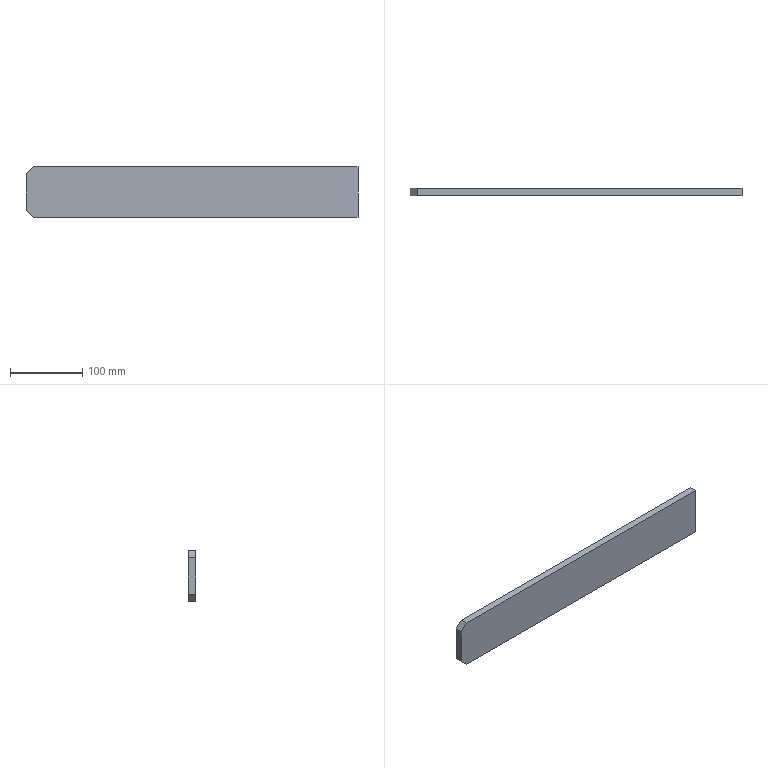Part | STEP file | Positioning_id1102_x_t | 1 solid | 8 faces | box 460 x 10 x 70 mm | volume 321000 mm3 | plane 8
STEP:
#1=CARTESIAN_POINT('',(0.,0.,0.));
#2=DIRECTION('',(0.,0.,1.));
#3=DIRECTION('',(1.,0.,0.));
#4=AXIS2_PLACEMENT_3D('',#1,#2,#3);
#5=CARTESIAN_POINT('',(-1483.002,800.,162.466));
#6=VERTEX_POINT('',#5);
#7=CARTESIAN_POINT('',(-1493.002,800.,172.466));
#8=VERTEX_POINT('',#7);
#9=CARTESIAN_POINT('',(-1483.002,800.,162.466));
#10=DIRECTION('',(-0.7071,0.,0.7071));
#11=VECTOR('',#10,1.);
#12=LINE('',#9,#11);
#13=CARTESIAN_POINT('',(-1493.002,800.,172.466));
#14=DIRECTION('',(0.7071,0.,0.7071));
#15=DIRECTION('',(-0.7071,0.,0.7071));
#16=AXIS2_PLACEMENT_3D('',#13,#14,#15);
#17=PLANE('',#16);
#18=CARTESIAN_POINT('',(-14.142,0.));
#19=DIRECTION('',(1.,0.));
#20=VECTOR('',#19,1.);
#21=LINE('',#18,#20);
#22=(GEOMETRIC_REPRESENTATION_CONTEXT(2)PARAMETRIC_REPRESENTATION_CONTEXT()REPRESENTATION_CONTEXT('',''));
#23=DEFINITIONAL_REPRESENTATION('',(#21),#22);
#24=PCURVE('',#17,#23);
#25=CARTESIAN_POINT('',(-1238.002,800.,197.466));
#26=DIRECTION('',(0.,-1.,0.));
#27=DIRECTION('',(0.,0.,1.));
#28=AXIS2_PLACEMENT_3D('',#25,#26,#27);
#29=PLANE('',#28);
#30=CARTESIAN_POINT('',(-35.,245.));
#31=DIRECTION('',(0.7071,0.7071));
#32=VECTOR('',#31,1.);
#33=LINE('',#30,#32);
#34=(GEOMETRIC_REPRESENTATION_CONTEXT(2)PARAMETRIC_REPRESENTATION_CONTEXT()REPRESENTATION_CONTEXT('',''));
#35=DEFINITIONAL_REPRESENTATION('',(#33),#34);
#36=PCURVE('',#29,#35);
#37=SURFACE_CURVE('',#12,(#24,#36),.PCURVE_S1.);
#38=EDGE_CURVE('',#6,#8,#37,.T.);
#39=ORIENTED_EDGE('',*,*,#38,.T.);
#40=CARTESIAN_POINT('',(-1493.002,810.,172.466));
#41=VERTEX_POINT('',#40);
#42=CARTESIAN_POINT('',(-1493.002,800.,172.466));
#43=DIRECTION('',(0.,1.,0.));
#44=VECTOR('',#43,1.);
#45=LINE('',#42,#44);
#46=CARTESIAN_POINT('',(0.,0.));
#47=DIRECTION('',(0.,-1.));
#48=VECTOR('',#47,1.);
#49=LINE('',#46,#48);
#50=(GEOMETRIC_REPRESENTATION_CONTEXT(2)PARAMETRIC_REPRESENTATION_CONTEXT()REPRESENTATION_CONTEXT('',''));
#51=DEFINITIONAL_REPRESENTATION('',(#49),#50);
#52=PCURVE('',#17,#51);
#53=CARTESIAN_POINT('',(-1493.002,800.,197.466));
#54=DIRECTION('',(-1.,0.,0.));
#55=DIRECTION('',(0.,-1.,0.));
#56=AXIS2_PLACEMENT_3D('',#53,#54,#55);
#57=PLANE('',#56);
#58=CARTESIAN_POINT('',(0.,-25.));
#59=DIRECTION('',(-1.,0.));
#60=VECTOR('',#59,1.);
#61=LINE('',#58,#60);
#62=(GEOMETRIC_REPRESENTATION_CONTEXT(2)PARAMETRIC_REPRESENTATION_CONTEXT()REPRESENTATION_CONTEXT('',''));
#63=DEFINITIONAL_REPRESENTATION('',(#61),#62);
#64=PCURVE('',#57,#63);
#65=SURFACE_CURVE('',#45,(#52,#64),.PCURVE_S1.);
#66=EDGE_CURVE('',#8,#41,#65,.T.);
#67=ORIENTED_EDGE('',*,*,#66,.T.);
#68=CARTESIAN_POINT('',(-1483.002,810.,162.466));
#69=VERTEX_POINT('',#68);
#70=CARTESIAN_POINT('',(-1493.002,810.,172.466));
#71=DIRECTION('',(0.7071,0.,-0.7071));
#72=VECTOR('',#71,1.);
#73=LINE('',#70,#72);
#74=CARTESIAN_POINT('',(0.,-10.));
#75=DIRECTION('',(-1.,0.));
#76=VECTOR('',#75,1.);
#77=LINE('',#74,#76);
#78=(GEOMETRIC_REPRESENTATION_CONTEXT(2)PARAMETRIC_REPRESENTATION_CONTEXT()REPRESENTATION_CONTEXT('',''));
#79=DEFINITIONAL_REPRESENTATION('',(#77),#78);
#80=PCURVE('',#17,#79);
#81=CARTESIAN_POINT('',(-1238.002,810.,197.466));
#82=DIRECTION('',(0.,1.,0.));
#83=DIRECTION('',(0.,0.,-1.));
#84=AXIS2_PLACEMENT_3D('',#81,#82,#83);
#85=PLANE('',#84);
#86=CARTESIAN_POINT('',(25.,255.));
#87=DIRECTION('',(0.7071,-0.7071));
#88=VECTOR('',#87,1.);
#89=LINE('',#86,#88);
#90=(GEOMETRIC_REPRESENTATION_CONTEXT(2)PARAMETRIC_REPRESENTATION_CONTEXT()REPRESENTATION_CONTEXT('',''));
#91=DEFINITIONAL_REPRESENTATION('',(#89),#90);
#92=PCURVE('',#85,#91);
#93=SURFACE_CURVE('',#73,(#80,#92),.PCURVE_S1.);
#94=EDGE_CURVE('',#41,#69,#93,.T.);
#95=ORIENTED_EDGE('',*,*,#94,.T.);
#96=CARTESIAN_POINT('',(-1483.002,810.,162.466));
#97=DIRECTION('',(0.,-1.,0.));
#98=VECTOR('',#97,1.);
#99=LINE('',#96,#98);
#100=CARTESIAN_POINT('',(-14.142,-10.));
#101=DIRECTION('',(0.,1.));
#102=VECTOR('',#101,1.);
#103=LINE('',#100,#102);
#104=(GEOMETRIC_REPRESENTATION_CONTEXT(2)PARAMETRIC_REPRESENTATION_CONTEXT()REPRESENTATION_CONTEXT('',''));
#105=DEFINITIONAL_REPRESENTATION('',(#103),#104);
#106=PCURVE('',#17,#105);
#107=CARTESIAN_POINT('',(-1238.002,800.,162.466));
#108=DIRECTION('',(0.,0.,-1.));
#109=DIRECTION('',(0.,-1.,0.));
#110=AXIS2_PLACEMENT_3D('',#107,#108,#109);
#111=PLANE('',#110);
#112=CARTESIAN_POINT('',(-10.,245.));
#113=DIRECTION('',(1.,0.));
#114=VECTOR('',#113,1.);
#115=LINE('',#112,#114);
#116=(GEOMETRIC_REPRESENTATION_CONTEXT(2)PARAMETRIC_REPRESENTATION_CONTEXT()REPRESENTATION_CONTEXT('',''));
#117=DEFINITIONAL_REPRESENTATION('',(#115),#116);
#118=PCURVE('',#111,#117);
#119=SURFACE_CURVE('',#99,(#106,#118),.PCURVE_S1.);
#120=EDGE_CURVE('',#69,#6,#119,.T.);
#121=ORIENTED_EDGE('',*,*,#120,.T.);
#122=EDGE_LOOP('',(#39,#67,#95,#121));
#123=FACE_BOUND('',#122,.T.);
#124=ADVANCED_FACE('',(#123),#17,.F.);
#125=CARTESIAN_POINT('',(-1493.002,800.,222.466));
#126=VERTEX_POINT('',#125);
#127=CARTESIAN_POINT('',(-1483.002,800.,232.466));
#128=VERTEX_POINT('',#127);
#129=CARTESIAN_POINT('',(-1493.002,800.,222.466));
#130=DIRECTION('',(0.7071,0.,0.7071));
#131=VECTOR('',#130,1.);
#132=LINE('',#129,#131);
#133=CARTESIAN_POINT('',(-1483.002,800.,232.466));
#134=DIRECTION('',(0.7071,0.,-0.7071));
#135=DIRECTION('',(0.7071,0.,0.7071));
#136=AXIS2_PLACEMENT_3D('',#133,#134,#135);
#137=PLANE('',#136);
#138=CARTESIAN_POINT('',(-14.142,0.));
#139=DIRECTION('',(1.,0.));
#140=VECTOR('',#139,1.);
#141=LINE('',#138,#140);
#142=(GEOMETRIC_REPRESENTATION_CONTEXT(2)PARAMETRIC_REPRESENTATION_CONTEXT()REPRESENTATION_CONTEXT('',''));
#143=DEFINITIONAL_REPRESENTATION('',(#141),#142);
#144=PCURVE('',#137,#143);
#145=CARTESIAN_POINT('',(25.,255.));
#146=DIRECTION('',(0.7071,-0.7071));
#147=VECTOR('',#146,1.);
#148=LINE('',#145,#147);
#149=(GEOMETRIC_REPRESENTATION_CONTEXT(2)PARAMETRIC_REPRESENTATION_CONTEXT()REPRESENTATION_CONTEXT('',''));
#150=DEFINITIONAL_REPRESENTATION('',(#148),#149);
#151=PCURVE('',#29,#150);
#152=SURFACE_CURVE('',#132,(#144,#151),.PCURVE_S1.);
#153=EDGE_CURVE('',#126,#128,#152,.T.);
#154=ORIENTED_EDGE('',*,*,#153,.T.);
#155=CARTESIAN_POINT('',(-1483.002,810.,232.466));
#156=VERTEX_POINT('',#155);
#157=CARTESIAN_POINT('',(-1483.002,800.,232.466));
#158=DIRECTION('',(0.,1.,0.));
#159=VECTOR('',#158,1.);
#160=LINE('',#157,#159);
#161=CARTESIAN_POINT('',(0.,0.));
#162=DIRECTION('',(0.,-1.));
#163=VECTOR('',#162,1.);
#164=LINE('',#161,#163);
#165=(GEOMETRIC_REPRESENTATION_CONTEXT(2)PARAMETRIC_REPRESENTATION_CONTEXT()REPRESENTATION_CONTEXT('',''));
#166=DEFINITIONAL_REPRESENTATION('',(#164),#165);
#167=PCURVE('',#137,#166);
#168=CARTESIAN_POINT('',(-1238.002,800.,232.466));
#169=DIRECTION('',(0.,0.,1.));
#170=DIRECTION('',(0.,1.,0.));
#171=AXIS2_PLACEMENT_3D('',#168,#169,#170);
#172=PLANE('',#171);
#173=CARTESIAN_POINT('',(0.,245.));
#174=DIRECTION('',(1.,0.));
#175=VECTOR('',#174,1.);
#176=LINE('',#173,#175);
#177=(GEOMETRIC_REPRESENTATION_CONTEXT(2)PARAMETRIC_REPRESENTATION_CONTEXT()REPRESENTATION_CONTEXT('',''));
#178=DEFINITIONAL_REPRESENTATION('',(#176),#177);
#179=PCURVE('',#172,#178);
#180=SURFACE_CURVE('',#160,(#167,#179),.PCURVE_S1.);
#181=EDGE_CURVE('',#128,#156,#180,.T.);
#182=ORIENTED_EDGE('',*,*,#181,.T.);
#183=CARTESIAN_POINT('',(-1493.002,810.,222.466));
#184=VERTEX_POINT('',#183);
#185=CARTESIAN_POINT('',(-1483.002,810.,232.466));
#186=DIRECTION('',(-0.7071,0.,-0.7071));
#187=VECTOR('',#186,1.);
#188=LINE('',#185,#187);
#189=CARTESIAN_POINT('',(0.,-10.));
#190=DIRECTION('',(-1.,0.));
#191=VECTOR('',#190,1.);
#192=LINE('',#189,#191);
#193=(GEOMETRIC_REPRESENTATION_CONTEXT(2)PARAMETRIC_REPRESENTATION_CONTEXT()REPRESENTATION_CONTEXT('',''));
#194=DEFINITIONAL_REPRESENTATION('',(#192),#193);
#195=PCURVE('',#137,#194);
#196=CARTESIAN_POINT('',(-35.,245.));
#197=DIRECTION('',(0.7071,0.7071));
#198=VECTOR('',#197,1.);
#199=LINE('',#196,#198);
#200=(GEOMETRIC_REPRESENTATION_CONTEXT(2)PARAMETRIC_REPRESENTATION_CONTEXT()REPRESENTATION_CONTEXT('',''));
#201=DEFINITIONAL_REPRESENTATION('',(#199),#200);
#202=PCURVE('',#85,#201);
#203=SURFACE_CURVE('',#188,(#195,#202),.PCURVE_S1.);
#204=EDGE_CURVE('',#156,#184,#203,.T.);
#205=ORIENTED_EDGE('',*,*,#204,.T.);
#206=CARTESIAN_POINT('',(-1493.002,810.,222.466));
#207=DIRECTION('',(0.,-1.,0.));
#208=VECTOR('',#207,1.);
#209=LINE('',#206,#208);
#210=CARTESIAN_POINT('',(-14.142,-10.));
#211=DIRECTION('',(0.,1.));
#212=VECTOR('',#211,1.);
#213=LINE('',#210,#212);
#214=(GEOMETRIC_REPRESENTATION_CONTEXT(2)PARAMETRIC_REPRESENTATION_CONTEXT()REPRESENTATION_CONTEXT('',''));
#215=DEFINITIONAL_REPRESENTATION('',(#213),#214);
#216=PCURVE('',#137,#215);
#217=CARTESIAN_POINT('',(-10.,25.));
#218=DIRECTION('',(1.,0.));
#219=VECTOR('',#218,1.);
#220=LINE('',#217,#219);
#221=(GEOMETRIC_REPRESENTATION_CONTEXT(2)PARAMETRIC_REPRESENTATION_CONTEXT()REPRESENTATION_CONTEXT('',''));
#222=DEFINITIONAL_REPRESENTATION('',(#220),#221);
#223=PCURVE('',#57,#222);
#224=SURFACE_CURVE('',#209,(#216,#223),.PCURVE_S1.);
#225=EDGE_CURVE('',#184,#126,#224,.T.);
#226=ORIENTED_EDGE('',*,*,#225,.T.);
#227=EDGE_LOOP('',(#154,#182,#205,#226));
#228=FACE_BOUND('',#227,.T.);
#229=ADVANCED_FACE('',(#228),#137,.F.);
#230=CARTESIAN_POINT('',(-1033.002,800.,232.466));
#231=VERTEX_POINT('',#230);
#232=CARTESIAN_POINT('',(-1033.002,800.,232.466));
#233=DIRECTION('',(-1.,0.,0.));
#234=VECTOR('',#233,1.);
#235=LINE('',#232,#234);
#236=CARTESIAN_POINT('',(0.,-205.));
#237=DIRECTION('',(0.,1.));
#238=VECTOR('',#237,1.);
#239=LINE('',#236,#238);
#240=(GEOMETRIC_REPRESENTATION_CONTEXT(2)PARAMETRIC_REPRESENTATION_CONTEXT()REPRESENTATION_CONTEXT('',''));
#241=DEFINITIONAL_REPRESENTATION('',(#239),#240);
#242=PCURVE('',#172,#241);
#243=CARTESIAN_POINT('',(35.,-205.));
#244=DIRECTION('',(0.,1.));
#245=VECTOR('',#244,1.);
#246=LINE('',#243,#245);
#247=(GEOMETRIC_REPRESENTATION_CONTEXT(2)PARAMETRIC_REPRESENTATION_CONTEXT()REPRESENTATION_CONTEXT('',''));
#248=DEFINITIONAL_REPRESENTATION('',(#246),#247);
#249=PCURVE('',#29,#248);
#250=SURFACE_CURVE('',#235,(#242,#249),.PCURVE_S1.);
#251=EDGE_CURVE('',#231,#128,#250,.T.);
#252=ORIENTED_EDGE('',*,*,#251,.F.);
#253=CARTESIAN_POINT('',(-1033.002,810.,232.466));
#254=VERTEX_POINT('',#253);
#255=CARTESIAN_POINT('',(-1033.002,800.,232.466));
#256=DIRECTION('',(0.,1.,0.));
#257=VECTOR('',#256,1.);
#258=LINE('',#255,#257);
#259=CARTESIAN_POINT('',(0.,-205.));
#260=DIRECTION('',(1.,0.));
#261=VECTOR('',#260,1.);
#262=LINE('',#259,#261);
#263=(GEOMETRIC_REPRESENTATION_CONTEXT(2)PARAMETRIC_REPRESENTATION_CONTEXT()REPRESENTATION_CONTEXT('',''));
#264=DEFINITIONAL_REPRESENTATION('',(#262),#263);
#265=PCURVE('',#172,#264);
#266=CARTESIAN_POINT('',(-1033.002,800.,197.466));
#267=DIRECTION('',(1.,0.,0.));
#268=DIRECTION('',(0.,1.,0.));
#269=AXIS2_PLACEMENT_3D('',#266,#267,#268);
#270=PLANE('',#269);
#271=CARTESIAN_POINT('',(0.,35.));
#272=DIRECTION('',(1.,0.));
#273=VECTOR('',#272,1.);
#274=LINE('',#271,#273);
#275=(GEOMETRIC_REPRESENTATION_CONTEXT(2)PARAMETRIC_REPRESENTATION_CONTEXT()REPRESENTATION_CONTEXT('',''));
#276=DEFINITIONAL_REPRESENTATION('',(#274),#275);
#277=PCURVE('',#270,#276);
#278=SURFACE_CURVE('',#258,(#265,#277),.PCURVE_S1.);
#279=EDGE_CURVE('',#231,#254,#278,.T.);
#280=ORIENTED_EDGE('',*,*,#279,.T.);
#281=CARTESIAN_POINT('',(-1483.002,810.,232.466));
#282=DIRECTION('',(1.,0.,0.));
#283=VECTOR('',#282,1.);
#284=LINE('',#281,#283);
#285=CARTESIAN_POINT('',(10.,245.));
#286=DIRECTION('',(0.,-1.));
#287=VECTOR('',#286,1.);
#288=LINE('',#285,#287);
#289=(GEOMETRIC_REPRESENTATION_CONTEXT(2)PARAMETRIC_REPRESENTATION_CONTEXT()REPRESENTATION_CONTEXT('',''));
#290=DEFINITIONAL_REPRESENTATION('',(#288),#289);
#291=PCURVE('',#172,#290);
#292=CARTESIAN_POINT('',(-35.,245.));
#293=DIRECTION('',(0.,-1.));
#294=VECTOR('',#293,1.);
#295=LINE('',#292,#294);
#296=(GEOMETRIC_REPRESENTATION_CONTEXT(2)PARAMETRIC_REPRESENTATION_CONTEXT()REPRESENTATION_CONTEXT('',''));
#297=DEFINITIONAL_REPRESENTATION('',(#295),#296);
#298=PCURVE('',#85,#297);
#299=SURFACE_CURVE('',#284,(#291,#298),.PCURVE_S1.);
#300=EDGE_CURVE('',#156,#254,#299,.T.);
#301=ORIENTED_EDGE('',*,*,#300,.F.);
#302=ORIENTED_EDGE('',*,*,#181,.F.);
#303=EDGE_LOOP('',(#252,#280,#301,#302));
#304=FACE_BOUND('',#303,.T.);
#305=ADVANCED_FACE('',(#304),#172,.T.);
#306=CARTESIAN_POINT('',(-1033.002,800.,162.466));
#307=VERTEX_POINT('',#306);
#308=CARTESIAN_POINT('',(-1483.002,800.,162.466));
#309=DIRECTION('',(1.,0.,0.));
#310=VECTOR('',#309,1.);
#311=LINE('',#308,#310);
#312=CARTESIAN_POINT('',(-35.,245.));
#313=DIRECTION('',(0.,-1.));
#314=VECTOR('',#313,1.);
#315=LINE('',#312,#314);
#316=(GEOMETRIC_REPRESENTATION_CONTEXT(2)PARAMETRIC_REPRESENTATION_CONTEXT()REPRESENTATION_CONTEXT('',''));
#317=DEFINITIONAL_REPRESENTATION('',(#315),#316);
#318=PCURVE('',#29,#317);
#319=CARTESIAN_POINT('',(0.,245.));
#320=DIRECTION('',(0.,-1.));
#321=VECTOR('',#320,1.);
#322=LINE('',#319,#321);
#323=(GEOMETRIC_REPRESENTATION_CONTEXT(2)PARAMETRIC_REPRESENTATION_CONTEXT()REPRESENTATION_CONTEXT('',''));
#324=DEFINITIONAL_REPRESENTATION('',(#322),#323);
#325=PCURVE('',#111,#324);
#326=SURFACE_CURVE('',#311,(#318,#325),.PCURVE_S1.);
#327=EDGE_CURVE('',#6,#307,#326,.T.);
#328=ORIENTED_EDGE('',*,*,#327,.T.);
#329=CARTESIAN_POINT('',(-1033.002,800.,162.466));
#330=DIRECTION('',(0.,0.,1.));
#331=VECTOR('',#330,1.);
#332=LINE('',#329,#331);
#333=CARTESIAN_POINT('',(-35.,-205.));
#334=DIRECTION('',(1.,0.));
#335=VECTOR('',#334,1.);
#336=LINE('',#333,#335);
#337=(GEOMETRIC_REPRESENTATION_CONTEXT(2)PARAMETRIC_REPRESENTATION_CONTEXT()REPRESENTATION_CONTEXT('',''));
#338=DEFINITIONAL_REPRESENTATION('',(#336),#337);
#339=PCURVE('',#29,#338);
#340=CARTESIAN_POINT('',(0.,-35.));
#341=DIRECTION('',(0.,1.));
#342=VECTOR('',#341,1.);
#343=LINE('',#340,#342);
#344=(GEOMETRIC_REPRESENTATION_CONTEXT(2)PARAMETRIC_REPRESENTATION_CONTEXT()REPRESENTATION_CONTEXT('',''));
#345=DEFINITIONAL_REPRESENTATION('',(#343),#344);
#346=PCURVE('',#270,#345);
#347=SURFACE_CURVE('',#332,(#339,#346),.PCURVE_S1.);
#348=EDGE_CURVE('',#307,#231,#347,.T.);
#349=ORIENTED_EDGE('',*,*,#348,.T.);
#350=ORIENTED_EDGE('',*,*,#251,.T.);
#351=ORIENTED_EDGE('',*,*,#153,.F.);
#352=CARTESIAN_POINT('',(-1493.002,800.,222.466));
#353=DIRECTION('',(0.,0.,-1.));
#354=VECTOR('',#353,1.);
#355=LINE('',#352,#354);
#356=CARTESIAN_POINT('',(25.,255.));
#357=DIRECTION('',(-1.,0.));
#358=VECTOR('',#357,1.);
#359=LINE('',#356,#358);
#360=(GEOMETRIC_REPRESENTATION_CONTEXT(2)PARAMETRIC_REPRESENTATION_CONTEXT()REPRESENTATION_CONTEXT('',''));
#361=DEFINITIONAL_REPRESENTATION('',(#359),#360);
#362=PCURVE('',#29,#361);
#363=CARTESIAN_POINT('',(0.,25.));
#364=DIRECTION('',(0.,-1.));
#365=VECTOR('',#364,1.);
#366=LINE('',#363,#365);
#367=(GEOMETRIC_REPRESENTATION_CONTEXT(2)PARAMETRIC_REPRESENTATION_CONTEXT()REPRESENTATION_CONTEXT('',''));
#368=DEFINITIONAL_REPRESENTATION('',(#366),#367);
#369=PCURVE('',#57,#368);
#370=SURFACE_CURVE('',#355,(#362,#369),.PCURVE_S1.);
#371=EDGE_CURVE('',#126,#8,#370,.T.);
#372=ORIENTED_EDGE('',*,*,#371,.T.);
#373=ORIENTED_EDGE('',*,*,#38,.F.);
#374=EDGE_LOOP('',(#328,#349,#350,#351,#372,#373));
#375=FACE_BOUND('',#374,.T.);
#376=ADVANCED_FACE('',(#375),#29,.T.);
#377=CARTESIAN_POINT('',(-1493.002,810.,172.466));
#378=DIRECTION('',(0.,0.,1.));
#379=VECTOR('',#378,1.);
#380=LINE('',#377,#379);
#381=CARTESIAN_POINT('',(-10.,-25.));
#382=DIRECTION('',(0.,1.));
#383=VECTOR('',#382,1.);
#384=LINE('',#381,#383);
#385=(GEOMETRIC_REPRESENTATION_CONTEXT(2)PARAMETRIC_REPRESENTATION_CONTEXT()REPRESENTATION_CONTEXT('',''));
#386=DEFINITIONAL_REPRESENTATION('',(#384),#385);
#387=PCURVE('',#57,#386);
#388=CARTESIAN_POINT('',(25.,255.));
#389=DIRECTION('',(-1.,0.));
#390=VECTOR('',#389,1.);
#391=LINE('',#388,#390);
#392=(GEOMETRIC_REPRESENTATION_CONTEXT(2)PARAMETRIC_REPRESENTATION_CONTEXT()REPRESENTATION_CONTEXT('',''));
#393=DEFINITIONAL_REPRESENTATION('',(#391),#392);
#394=PCURVE('',#85,#393);
#395=SURFACE_CURVE('',#380,(#387,#394),.PCURVE_S1.);
#396=EDGE_CURVE('',#41,#184,#395,.T.);
#397=ORIENTED_EDGE('',*,*,#396,.F.);
#398=ORIENTED_EDGE('',*,*,#66,.F.);
#399=ORIENTED_EDGE('',*,*,#371,.F.);
#400=ORIENTED_EDGE('',*,*,#225,.F.);
#401=EDGE_LOOP('',(#397,#398,#399,#400));
#402=FACE_BOUND('',#401,.T.);
#403=ADVANCED_FACE('',(#402),#57,.T.);
#404=CARTESIAN_POINT('',(-1033.002,810.,162.466));
#405=VERTEX_POINT('',#404);
#406=CARTESIAN_POINT('',(-1033.002,800.,162.466));
#407=DIRECTION('',(0.,1.,0.));
#408=VECTOR('',#407,1.);
#409=LINE('',#406,#408);
#410=CARTESIAN_POINT('',(0.,-205.));
#411=DIRECTION('',(-1.,0.));
#412=VECTOR('',#411,1.);
#413=LINE('',#410,#412);
#414=(GEOMETRIC_REPRESENTATION_CONTEXT(2)PARAMETRIC_REPRESENTATION_CONTEXT()REPRESENTATION_CONTEXT('',''));
#415=DEFINITIONAL_REPRESENTATION('',(#413),#414);
#416=PCURVE('',#111,#415);
#417=CARTESIAN_POINT('',(0.,-35.));
#418=DIRECTION('',(1.,0.));
#419=VECTOR('',#418,1.);
#420=LINE('',#417,#419);
#421=(GEOMETRIC_REPRESENTATION_CONTEXT(2)PARAMETRIC_REPRESENTATION_CONTEXT()REPRESENTATION_CONTEXT('',''));
#422=DEFINITIONAL_REPRESENTATION('',(#420),#421);
#423=PCURVE('',#270,#422);
#424=SURFACE_CURVE('',#409,(#416,#423),.PCURVE_S1.);
#425=EDGE_CURVE('',#307,#405,#424,.T.);
#426=ORIENTED_EDGE('',*,*,#425,.F.);
#427=ORIENTED_EDGE('',*,*,#327,.F.);
#428=ORIENTED_EDGE('',*,*,#120,.F.);
#429=CARTESIAN_POINT('',(-1033.002,810.,162.466));
#430=DIRECTION('',(-1.,0.,0.));
#431=VECTOR('',#430,1.);
#432=LINE('',#429,#431);
#433=CARTESIAN_POINT('',(-10.,-205.));
#434=DIRECTION('',(0.,1.));
#435=VECTOR('',#434,1.);
#436=LINE('',#433,#435);
#437=(GEOMETRIC_REPRESENTATION_CONTEXT(2)PARAMETRIC_REPRESENTATION_CONTEXT()REPRESENTATION_CONTEXT('',''));
#438=DEFINITIONAL_REPRESENTATION('',(#436),#437);
#439=PCURVE('',#111,#438);
#440=CARTESIAN_POINT('',(35.,-205.));
#441=DIRECTION('',(0.,1.));
#442=VECTOR('',#441,1.);
#443=LINE('',#440,#442);
#444=(GEOMETRIC_REPRESENTATION_CONTEXT(2)PARAMETRIC_REPRESENTATION_CONTEXT()REPRESENTATION_CONTEXT('',''));
#445=DEFINITIONAL_REPRESENTATION('',(#443),#444);
#446=PCURVE('',#85,#445);
#447=SURFACE_CURVE('',#432,(#439,#446),.PCURVE_S1.);
#448=EDGE_CURVE('',#405,#69,#447,.T.);
#449=ORIENTED_EDGE('',*,*,#448,.F.);
#450=EDGE_LOOP('',(#426,#427,#428,#449));
#451=FACE_BOUND('',#450,.T.);
#452=ADVANCED_FACE('',(#451),#111,.T.);
#453=ORIENTED_EDGE('',*,*,#348,.F.);
#454=ORIENTED_EDGE('',*,*,#425,.T.);
#455=CARTESIAN_POINT('',(-1033.002,810.,232.466));
#456=DIRECTION('',(0.,0.,-1.));
#457=VECTOR('',#456,1.);
#458=LINE('',#455,#457);
#459=CARTESIAN_POINT('',(10.,35.));
#460=DIRECTION('',(0.,-1.));
#461=VECTOR('',#460,1.);
#462=LINE('',#459,#461);
#463=(GEOMETRIC_REPRESENTATION_CONTEXT(2)PARAMETRIC_REPRESENTATION_CONTEXT()REPRESENTATION_CONTEXT('',''));
#464=DEFINITIONAL_REPRESENTATION('',(#462),#463);
#465=PCURVE('',#270,#464);
#466=CARTESIAN_POINT('',(-35.,-205.));
#467=DIRECTION('',(1.,0.));
#468=VECTOR('',#467,1.);
#469=LINE('',#466,#468);
#470=(GEOMETRIC_REPRESENTATION_CONTEXT(2)PARAMETRIC_REPRESENTATION_CONTEXT()REPRESENTATION_CONTEXT('',''));
#471=DEFINITIONAL_REPRESENTATION('',(#469),#470);
#472=PCURVE('',#85,#471);
#473=SURFACE_CURVE('',#458,(#465,#472),.PCURVE_S1.);
#474=EDGE_CURVE('',#254,#405,#473,.T.);
#475=ORIENTED_EDGE('',*,*,#474,.F.);
#476=ORIENTED_EDGE('',*,*,#279,.F.);
#477=EDGE_LOOP('',(#453,#454,#475,#476));
#478=FACE_BOUND('',#477,.T.);
#479=ADVANCED_FACE('',(#478),#270,.T.);
#480=ORIENTED_EDGE('',*,*,#474,.T.);
#481=ORIENTED_EDGE('',*,*,#448,.T.);
#482=ORIENTED_EDGE('',*,*,#94,.F.);
#483=ORIENTED_EDGE('',*,*,#396,.T.);
#484=ORIENTED_EDGE('',*,*,#204,.F.);
#485=ORIENTED_EDGE('',*,*,#300,.T.);
#486=EDGE_LOOP('',(#480,#481,#482,#483,#484,#485));
#487=FACE_BOUND('',#486,.T.);
#488=ADVANCED_FACE('',(#487),#85,.T.);
#489=CLOSED_SHELL('',(#124,#229,#305,#376,#403,#452,#479,#488));
#490=MANIFOLD_SOLID_BREP('',#489);
#491=(LENGTH_UNIT()NAMED_UNIT(*)SI_UNIT(.MILLI.,.METRE.));
#492=UNCERTAINTY_MEASURE_WITH_UNIT(LENGTH_MEASURE(0.0000001),#491,'','');
#493=(NAMED_UNIT(*)PLANE_ANGLE_UNIT()SI_UNIT($,.RADIAN.));
#494=(NAMED_UNIT(*)SI_UNIT($,.STERADIAN.)SOLID_ANGLE_UNIT());
#495=(GEOMETRIC_REPRESENTATION_CONTEXT(3)GLOBAL_UNCERTAINTY_ASSIGNED_CONTEXT((#492))GLOBAL_UNIT_ASSIGNED_CONTEXT((#491,#493,#494))REPRESENTATION_CONTEXT('',''));
#496=ADVANCED_BREP_SHAPE_REPRESENTATION('',(#4,#490),#495);